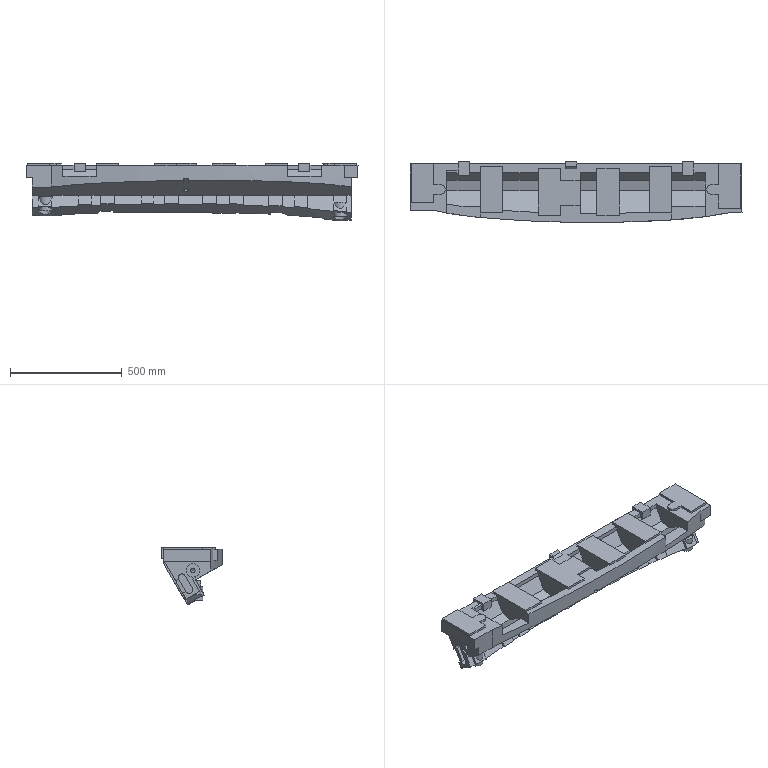Part | NX | features MAIN_BODY 2 | 1 solid | 268 faces | box 1487 x 272.345 x 259.68 mm | volume 40346521 mm3 | plane 227 | cylinder 26 | spline 11 | cone 4 | commonest cylinder face diameters 60 x9 20 x7 32 x6 40 x2 45 x2